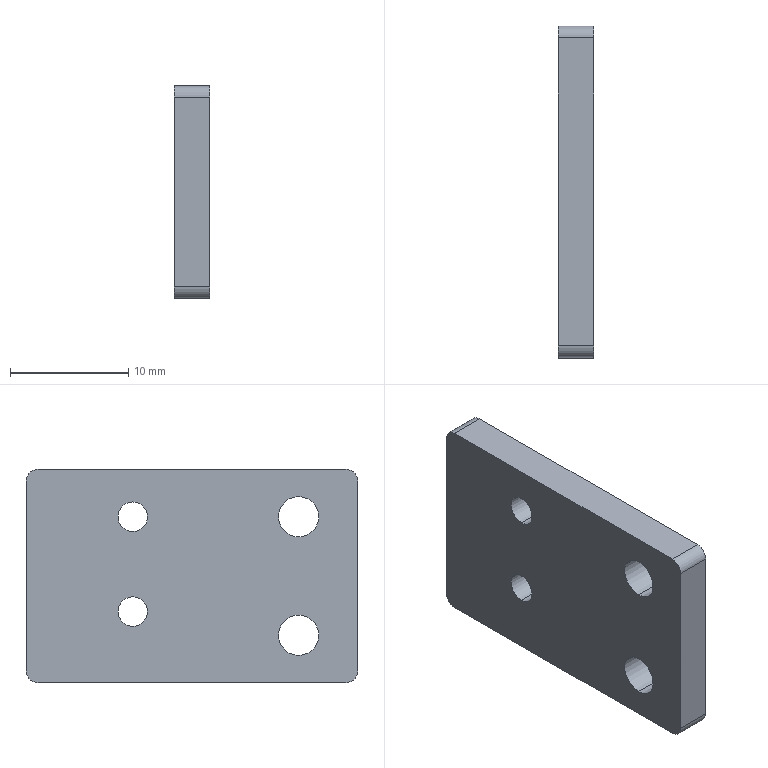Part | NX | features BREP 1 | 1 solid | 18 faces | box 3 x 28 x 18 mm | volume 1425 mm3 | cylinder 12 | plane 6 | commonest cylinder face diameters 2 x4 2.5 x4 3.4 x4
STEP:
#1=CARTESIAN_POINT('',(-3.,28.,-8.));
#2=VERTEX_POINT('',#1);
#3=CARTESIAN_POINT('',(-3.,27.,-9.));
#4=VERTEX_POINT('',#3);
#5=CARTESIAN_POINT('',(-3.,27.,-8.));
#6=DIRECTION('',(-1.,0.,0.));
#7=DIRECTION('',(0.,1.,0.));
#8=AXIS2_PLACEMENT_3D('',#5,#6,#7);
#9=CIRCLE('',#8,1.);
#10=EDGE_CURVE('',#2,#4,#9,.T.);
#11=ORIENTED_EDGE('',*,*,#10,.F.);
#12=CARTESIAN_POINT('',(0.,28.,-8.));
#13=VERTEX_POINT('',#12);
#14=CARTESIAN_POINT('',(-3.,28.,-8.));
#15=DIRECTION('',(-1.,0.,0.));
#16=VECTOR('',#15,1000.);
#17=LINE('',#14,#16);
#18=EDGE_CURVE('',#13,#2,#17,.T.);
#19=ORIENTED_EDGE('',*,*,#18,.F.);
#20=CARTESIAN_POINT('',(0.,27.,-9.));
#21=VERTEX_POINT('',#20);
#22=CARTESIAN_POINT('',(0.,27.,-8.));
#23=DIRECTION('',(1.,0.,0.));
#24=DIRECTION('',(0.,1.,0.));
#25=AXIS2_PLACEMENT_3D('',#22,#23,#24);
#26=CIRCLE('',#25,1.);
#27=EDGE_CURVE('',#21,#13,#26,.T.);
#28=ORIENTED_EDGE('',*,*,#27,.F.);
#29=CARTESIAN_POINT('',(0.,27.,-9.));
#30=DIRECTION('',(1.,0.,0.));
#31=VECTOR('',#30,1000.);
#32=LINE('',#29,#31);
#33=EDGE_CURVE('',#4,#21,#32,.T.);
#34=ORIENTED_EDGE('',*,*,#33,.F.);
#35=EDGE_LOOP('',(#11,#19,#28,#34));
#36=FACE_BOUND('',#35,.T.);
#37=CARTESIAN_POINT('',(0.,27.,-8.));
#38=DIRECTION('',(1.,0.,0.));
#39=DIRECTION('',(0.,0.,-1.));
#40=AXIS2_PLACEMENT_3D('',#37,#38,#39);
#41=CYLINDRICAL_SURFACE('',#40,1.);
#42=ADVANCED_FACE('',(#36),#41,.T.);
#43=CARTESIAN_POINT('',(-3.,27.,9.));
#44=VERTEX_POINT('',#43);
#45=CARTESIAN_POINT('',(-3.,28.,8.));
#46=VERTEX_POINT('',#45);
#47=CARTESIAN_POINT('',(-3.,27.,8.));
#48=DIRECTION('',(-1.,0.,0.));
#49=DIRECTION('',(0.,1.,0.));
#50=AXIS2_PLACEMENT_3D('',#47,#48,#49);
#51=CIRCLE('',#50,1.);
#52=EDGE_CURVE('',#44,#46,#51,.T.);
#53=ORIENTED_EDGE('',*,*,#52,.F.);
#54=CARTESIAN_POINT('',(0.,27.,9.));
#55=VERTEX_POINT('',#54);
#56=CARTESIAN_POINT('',(-3.,27.,9.));
#57=DIRECTION('',(-1.,0.,0.));
#58=VECTOR('',#57,1000.);
#59=LINE('',#56,#58);
#60=EDGE_CURVE('',#55,#44,#59,.T.);
#61=ORIENTED_EDGE('',*,*,#60,.F.);
#62=CARTESIAN_POINT('',(0.,28.,8.));
#63=VERTEX_POINT('',#62);
#64=CARTESIAN_POINT('',(0.,27.,8.));
#65=DIRECTION('',(1.,0.,0.));
#66=DIRECTION('',(0.,1.,0.));
#67=AXIS2_PLACEMENT_3D('',#64,#65,#66);
#68=CIRCLE('',#67,1.);
#69=EDGE_CURVE('',#63,#55,#68,.T.);
#70=ORIENTED_EDGE('',*,*,#69,.F.);
#71=CARTESIAN_POINT('',(0.,28.,8.));
#72=DIRECTION('',(1.,0.,0.));
#73=VECTOR('',#72,1000.);
#74=LINE('',#71,#73);
#75=EDGE_CURVE('',#46,#63,#74,.T.);
#76=ORIENTED_EDGE('',*,*,#75,.F.);
#77=EDGE_LOOP('',(#53,#61,#70,#76));
#78=FACE_BOUND('',#77,.T.);
#79=CARTESIAN_POINT('',(-3.,27.,8.));
#80=DIRECTION('',(-1.,0.,0.));
#81=DIRECTION('',(0.,0.,1.));
#82=AXIS2_PLACEMENT_3D('',#79,#80,#81);
#83=CYLINDRICAL_SURFACE('',#82,1.);
#84=ADVANCED_FACE('',(#78),#83,.T.);
#85=CARTESIAN_POINT('',(0.,0.,-8.));
#86=VERTEX_POINT('',#85);
#87=CARTESIAN_POINT('',(0.,1.,-9.));
#88=VERTEX_POINT('',#87);
#89=CARTESIAN_POINT('',(0.,1.,-8.));
#90=DIRECTION('',(1.,0.,0.));
#91=DIRECTION('',(0.,1.,0.));
#92=AXIS2_PLACEMENT_3D('',#89,#90,#91);
#93=CIRCLE('',#92,1.);
#94=EDGE_CURVE('',#86,#88,#93,.T.);
#95=ORIENTED_EDGE('',*,*,#94,.F.);
#96=CARTESIAN_POINT('',(-3.,0.,-8.));
#97=VERTEX_POINT('',#96);
#98=CARTESIAN_POINT('',(0.,0.,-8.));
#99=DIRECTION('',(1.,0.,0.));
#100=VECTOR('',#99,1000.);
#101=LINE('',#98,#100);
#102=EDGE_CURVE('',#97,#86,#101,.T.);
#103=ORIENTED_EDGE('',*,*,#102,.F.);
#104=CARTESIAN_POINT('',(-3.,1.,-9.));
#105=VERTEX_POINT('',#104);
#106=CARTESIAN_POINT('',(-3.,1.,-8.));
#107=DIRECTION('',(-1.,0.,0.));
#108=DIRECTION('',(0.,1.,0.));
#109=AXIS2_PLACEMENT_3D('',#106,#107,#108);
#110=CIRCLE('',#109,1.);
#111=EDGE_CURVE('',#105,#97,#110,.T.);
#112=ORIENTED_EDGE('',*,*,#111,.F.);
#113=CARTESIAN_POINT('',(0.,1.,-9.));
#114=DIRECTION('',(-1.,0.,0.));
#115=VECTOR('',#114,1000.);
#116=LINE('',#113,#115);
#117=EDGE_CURVE('',#88,#105,#116,.T.);
#118=ORIENTED_EDGE('',*,*,#117,.F.);
#119=EDGE_LOOP('',(#95,#103,#112,#118));
#120=FACE_BOUND('',#119,.T.);
#121=CARTESIAN_POINT('',(0.,1.,-8.));
#122=DIRECTION('',(-1.,0.,0.));
#123=DIRECTION('',(0.,0.,1.));
#124=AXIS2_PLACEMENT_3D('',#121,#122,#123);
#125=CYLINDRICAL_SURFACE('',#124,1.);
#126=ADVANCED_FACE('',(#120),#125,.T.);
#127=CARTESIAN_POINT('',(0.,1.,9.));
#128=VERTEX_POINT('',#127);
#129=CARTESIAN_POINT('',(0.,0.,8.));
#130=VERTEX_POINT('',#129);
#131=CARTESIAN_POINT('',(0.,1.,8.));
#132=DIRECTION('',(1.,0.,0.));
#133=DIRECTION('',(0.,1.,0.));
#134=AXIS2_PLACEMENT_3D('',#131,#132,#133);
#135=CIRCLE('',#134,1.);
#136=EDGE_CURVE('',#128,#130,#135,.T.);
#137=ORIENTED_EDGE('',*,*,#136,.F.);
#138=CARTESIAN_POINT('',(-3.,1.,9.));
#139=VERTEX_POINT('',#138);
#140=CARTESIAN_POINT('',(0.,1.,9.));
#141=DIRECTION('',(1.,0.,0.));
#142=VECTOR('',#141,1000.);
#143=LINE('',#140,#142);
#144=EDGE_CURVE('',#139,#128,#143,.T.);
#145=ORIENTED_EDGE('',*,*,#144,.F.);
#146=CARTESIAN_POINT('',(-3.,0.,8.));
#147=VERTEX_POINT('',#146);
#148=CARTESIAN_POINT('',(-3.,1.,8.));
#149=DIRECTION('',(-1.,0.,0.));
#150=DIRECTION('',(0.,1.,0.));
#151=AXIS2_PLACEMENT_3D('',#148,#149,#150);
#152=CIRCLE('',#151,1.);
#153=EDGE_CURVE('',#147,#139,#152,.T.);
#154=ORIENTED_EDGE('',*,*,#153,.F.);
#155=CARTESIAN_POINT('',(-3.,0.,8.));
#156=DIRECTION('',(-1.,0.,0.));
#157=VECTOR('',#156,1000.);
#158=LINE('',#155,#157);
#159=EDGE_CURVE('',#130,#147,#158,.T.);
#160=ORIENTED_EDGE('',*,*,#159,.F.);
#161=EDGE_LOOP('',(#137,#145,#154,#160));
#162=FACE_BOUND('',#161,.T.);
#163=CARTESIAN_POINT('',(0.,1.,8.));
#164=DIRECTION('',(1.,0.,0.));
#165=DIRECTION('',(0.,0.,-1.));
#166=AXIS2_PLACEMENT_3D('',#163,#164,#165);
#167=CYLINDRICAL_SURFACE('',#166,1.);
#168=ADVANCED_FACE('',(#162),#167,.T.);
#169=CARTESIAN_POINT('',(-3.,5.,-6.7));
#170=VERTEX_POINT('',#169);
#171=CARTESIAN_POINT('',(0.,5.,-6.7));
#172=VERTEX_POINT('',#171);
#173=CARTESIAN_POINT('',(-3.,5.,-6.7));
#174=DIRECTION('',(-1.,0.,0.));
#175=VECTOR('',#174,1000.);
#176=LINE('',#173,#175);
#177=EDGE_CURVE('',#170,#172,#176,.F.);
#178=ORIENTED_EDGE('',*,*,#177,.T.);
#179=CARTESIAN_POINT('',(0.,5.,-3.3));
#180=VERTEX_POINT('',#179);
#181=CARTESIAN_POINT('',(0.,5.,-5.));
#182=DIRECTION('',(-1.,0.,0.));
#183=DIRECTION('',(0.,0.,1.));
#184=AXIS2_PLACEMENT_3D('',#181,#182,#183);
#185=CIRCLE('',#184,1.7);
#186=EDGE_CURVE('',#180,#172,#185,.T.);
#187=ORIENTED_EDGE('',*,*,#186,.F.);
#188=CARTESIAN_POINT('',(-3.,5.,-3.3));
#189=VERTEX_POINT('',#188);
#190=CARTESIAN_POINT('',(-3.,5.,-3.3));
#191=DIRECTION('',(-1.,0.,0.));
#192=VECTOR('',#191,1000.);
#193=LINE('',#190,#192);
#194=EDGE_CURVE('',#189,#180,#193,.F.);
#195=ORIENTED_EDGE('',*,*,#194,.F.);
#196=CARTESIAN_POINT('',(-3.,5.,-5.));
#197=DIRECTION('',(-1.,0.,0.));
#198=DIRECTION('',(0.,0.,1.));
#199=AXIS2_PLACEMENT_3D('',#196,#197,#198);
#200=CIRCLE('',#199,1.7);
#201=EDGE_CURVE('',#189,#170,#200,.T.);
#202=ORIENTED_EDGE('',*,*,#201,.T.);
#203=EDGE_LOOP('',(#178,#187,#195,#202));
#204=FACE_BOUND('',#203,.T.);
#205=CARTESIAN_POINT('',(-3.,5.,-5.));
#206=DIRECTION('',(-1.,0.,0.));
#207=DIRECTION('',(0.,0.,1.));
#208=AXIS2_PLACEMENT_3D('',#205,#206,#207);
#209=CYLINDRICAL_SURFACE('',#208,1.7);
#210=ADVANCED_FACE('',(#204),#209,.F.);
#211=CARTESIAN_POINT('',(-3.,5.,3.3));
#212=VERTEX_POINT('',#211);
#213=CARTESIAN_POINT('',(0.,5.,3.3));
#214=VERTEX_POINT('',#213);
#215=CARTESIAN_POINT('',(-3.,5.,3.3));
#216=DIRECTION('',(-1.,0.,0.));
#217=VECTOR('',#216,1000.);
#218=LINE('',#215,#217);
#219=EDGE_CURVE('',#212,#214,#218,.F.);
#220=ORIENTED_EDGE('',*,*,#219,.T.);
#221=CARTESIAN_POINT('',(0.,5.,6.7));
#222=VERTEX_POINT('',#221);
#223=CARTESIAN_POINT('',(0.,5.,5.));
#224=DIRECTION('',(-1.,0.,0.));
#225=DIRECTION('',(0.,0.,1.));
#226=AXIS2_PLACEMENT_3D('',#223,#224,#225);
#227=CIRCLE('',#226,1.7);
#228=EDGE_CURVE('',#222,#214,#227,.T.);
#229=ORIENTED_EDGE('',*,*,#228,.F.);
#230=CARTESIAN_POINT('',(-3.,5.,6.7));
#231=VERTEX_POINT('',#230);
#232=CARTESIAN_POINT('',(-3.,5.,6.7));
#233=DIRECTION('',(-1.,0.,0.));
#234=VECTOR('',#233,1000.);
#235=LINE('',#232,#234);
#236=EDGE_CURVE('',#231,#222,#235,.F.);
#237=ORIENTED_EDGE('',*,*,#236,.F.);
#238=CARTESIAN_POINT('',(-3.,5.,5.));
#239=DIRECTION('',(-1.,0.,0.));
#240=DIRECTION('',(0.,0.,1.));
#241=AXIS2_PLACEMENT_3D('',#238,#239,#240);
#242=CIRCLE('',#241,1.7);
#243=EDGE_CURVE('',#231,#212,#242,.T.);
#244=ORIENTED_EDGE('',*,*,#243,.T.);
#245=EDGE_LOOP('',(#220,#229,#237,#244));
#246=FACE_BOUND('',#245,.T.);
#247=CARTESIAN_POINT('',(-3.,5.,5.));
#248=DIRECTION('',(-1.,0.,0.));
#249=DIRECTION('',(0.,0.,1.));
#250=AXIS2_PLACEMENT_3D('',#247,#248,#249);
#251=CYLINDRICAL_SURFACE('',#250,1.7);
#252=ADVANCED_FACE('',(#246),#251,.F.);
#253=CARTESIAN_POINT('',(-3.,19.,-4.25));
#254=VERTEX_POINT('',#253);
#255=CARTESIAN_POINT('',(0.,19.,-4.25));
#256=VERTEX_POINT('',#255);
#257=CARTESIAN_POINT('',(-3.,19.,-4.25));
#258=DIRECTION('',(-1.,0.,0.));
#259=VECTOR('',#258,1000.);
#260=LINE('',#257,#259);
#261=EDGE_CURVE('',#254,#256,#260,.F.);
#262=ORIENTED_EDGE('',*,*,#261,.T.);
#263=CARTESIAN_POINT('',(0.,19.,-1.75));
#264=VERTEX_POINT('',#263);
#265=CARTESIAN_POINT('',(0.,19.,-3.));
#266=DIRECTION('',(1.,0.,0.));
#267=DIRECTION('',(0.,1.,0.));
#268=AXIS2_PLACEMENT_3D('',#265,#266,#267);
#269=CIRCLE('',#268,1.25);
#270=EDGE_CURVE('',#256,#264,#269,.T.);
#271=ORIENTED_EDGE('',*,*,#270,.T.);
#272=CARTESIAN_POINT('',(-3.,19.,-1.75));
#273=VERTEX_POINT('',#272);
#274=CARTESIAN_POINT('',(-3.,19.,-1.75));
#275=DIRECTION('',(-1.,0.,0.));
#276=VECTOR('',#275,1000.);
#277=LINE('',#274,#276);
#278=EDGE_CURVE('',#273,#264,#277,.F.);
#279=ORIENTED_EDGE('',*,*,#278,.F.);
#280=CARTESIAN_POINT('',(-3.,19.,-3.));
#281=DIRECTION('',(-1.,0.,0.));
#282=DIRECTION('',(0.,0.,1.));
#283=AXIS2_PLACEMENT_3D('',#280,#281,#282);
#284=CIRCLE('',#283,1.25);
#285=EDGE_CURVE('',#273,#254,#284,.T.);
#286=ORIENTED_EDGE('',*,*,#285,.T.);
#287=EDGE_LOOP('',(#262,#271,#279,#286));
#288=FACE_BOUND('',#287,.T.);
#289=CARTESIAN_POINT('',(-3.,19.,-3.));
#290=DIRECTION('',(-1.,0.,0.));
#291=DIRECTION('',(0.,0.,1.));
#292=AXIS2_PLACEMENT_3D('',#289,#290,#291);
#293=CYLINDRICAL_SURFACE('',#292,1.25);
#294=ADVANCED_FACE('',(#288),#293,.F.);
#295=CARTESIAN_POINT('',(-3.,19.,3.75));
#296=VERTEX_POINT('',#295);
#297=CARTESIAN_POINT('',(0.,19.,3.75));
#298=VERTEX_POINT('',#297);
#299=CARTESIAN_POINT('',(-3.,19.,3.75));
#300=DIRECTION('',(-1.,0.,0.));
#301=VECTOR('',#300,1000.);
#302=LINE('',#299,#301);
#303=EDGE_CURVE('',#296,#298,#302,.F.);
#304=ORIENTED_EDGE('',*,*,#303,.T.);
#305=CARTESIAN_POINT('',(0.,19.,6.25));
#306=VERTEX_POINT('',#305);
#307=CARTESIAN_POINT('',(0.,19.,5.));
#308=DIRECTION('',(1.,0.,0.));
#309=DIRECTION('',(0.,1.,0.));
#310=AXIS2_PLACEMENT_3D('',#307,#308,#309);
#311=CIRCLE('',#310,1.25);
#312=EDGE_CURVE('',#298,#306,#311,.T.);
#313=ORIENTED_EDGE('',*,*,#312,.T.);
#314=CARTESIAN_POINT('',(-3.,19.,6.25));
#315=VERTEX_POINT('',#314);
#316=CARTESIAN_POINT('',(-3.,19.,6.25));
#317=DIRECTION('',(-1.,0.,0.));
#318=VECTOR('',#317,1000.);
#319=LINE('',#316,#318);
#320=EDGE_CURVE('',#315,#306,#319,.F.);
#321=ORIENTED_EDGE('',*,*,#320,.F.);
#322=CARTESIAN_POINT('',(-3.,19.,5.));
#323=DIRECTION('',(-1.,0.,0.));
#324=DIRECTION('',(0.,0.,1.));
#325=AXIS2_PLACEMENT_3D('',#322,#323,#324);
#326=CIRCLE('',#325,1.25);
#327=EDGE_CURVE('',#315,#296,#326,.T.);
#328=ORIENTED_EDGE('',*,*,#327,.T.);
#329=EDGE_LOOP('',(#304,#313,#321,#328));
#330=FACE_BOUND('',#329,.T.);
#331=CARTESIAN_POINT('',(-3.,19.,5.));
#332=DIRECTION('',(-1.,0.,0.));
#333=DIRECTION('',(0.,0.,1.));
#334=AXIS2_PLACEMENT_3D('',#331,#332,#333);
#335=CYLINDRICAL_SURFACE('',#334,1.25);
#336=ADVANCED_FACE('',(#330),#335,.F.);
#337=CARTESIAN_POINT('',(0.,28.,-9.));
#338=DIRECTION('',(0.,-1.,0.));
#339=VECTOR('',#338,1000.);
#340=LINE('',#337,#339);
#341=EDGE_CURVE('',#21,#88,#340,.T.);
#342=ORIENTED_EDGE('',*,*,#341,.T.);
#343=ORIENTED_EDGE('',*,*,#117,.T.);
#344=CARTESIAN_POINT('',(-3.,28.,-9.));
#345=DIRECTION('',(0.,-1.,0.));
#346=VECTOR('',#345,1000.);
#347=LINE('',#344,#346);
#348=EDGE_CURVE('',#4,#105,#347,.T.);
#349=ORIENTED_EDGE('',*,*,#348,.F.);
#350=ORIENTED_EDGE('',*,*,#33,.T.);
#351=EDGE_LOOP('',(#342,#343,#349,#350));
#352=FACE_BOUND('',#351,.T.);
#353=CARTESIAN_POINT('',(0.,0.,-9.));
#354=DIRECTION('',(0.,0.,-1.));
#355=DIRECTION('',(-1.,0.,0.));
#356=AXIS2_PLACEMENT_3D('',#353,#354,#355);
#357=PLANE('',#356);
#358=ADVANCED_FACE('',(#352),#357,.T.);
#359=CARTESIAN_POINT('',(-3.,28.,9.));
#360=DIRECTION('',(0.,-1.,0.));
#361=VECTOR('',#360,1000.);
#362=LINE('',#359,#361);
#363=EDGE_CURVE('',#44,#139,#362,.T.);
#364=ORIENTED_EDGE('',*,*,#363,.T.);
#365=ORIENTED_EDGE('',*,*,#144,.T.);
#366=CARTESIAN_POINT('',(0.,28.,9.));
#367=DIRECTION('',(0.,-1.,0.));
#368=VECTOR('',#367,1000.);
#369=LINE('',#366,#368);
#370=EDGE_CURVE('',#55,#128,#369,.T.);
#371=ORIENTED_EDGE('',*,*,#370,.F.);
#372=ORIENTED_EDGE('',*,*,#60,.T.);
#373=EDGE_LOOP('',(#364,#365,#371,#372));
#374=FACE_BOUND('',#373,.T.);
#375=CARTESIAN_POINT('',(0.,0.,9.));
#376=DIRECTION('',(0.,0.,-1.));
#377=DIRECTION('',(-1.,0.,0.));
#378=AXIS2_PLACEMENT_3D('',#375,#376,#377);
#379=PLANE('',#378);
#380=ADVANCED_FACE('',(#374),#379,.F.);
#381=CARTESIAN_POINT('',(-3.,28.,9.));
#382=DIRECTION('',(0.,0.,-1.));
#383=VECTOR('',#382,1000.);
#384=LINE('',#381,#383);
#385=EDGE_CURVE('',#46,#2,#384,.T.);
#386=ORIENTED_EDGE('',*,*,#385,.F.);
#387=ORIENTED_EDGE('',*,*,#75,.T.);
#388=CARTESIAN_POINT('',(0.,28.,9.));
#389=DIRECTION('',(0.,0.,-1.));
#390=VECTOR('',#389,1000.);
#391=LINE('',#388,#390);
#392=EDGE_CURVE('',#63,#13,#391,.T.);
#393=ORIENTED_EDGE('',*,*,#392,.T.);
#394=ORIENTED_EDGE('',*,*,#18,.T.);
#395=EDGE_LOOP('',(#386,#387,#393,#394));
#396=FACE_BOUND('',#395,.T.);
#397=CARTESIAN_POINT('',(-3.,28.,9.));
#398=DIRECTION('',(0.,1.,0.));
#399=DIRECTION('',(0.,0.,1.));
#400=AXIS2_PLACEMENT_3D('',#397,#398,#399);
#401=PLANE('',#400);
#402=ADVANCED_FACE('',(#396),#401,.T.);
#403=ORIENTED_EDGE('',*,*,#370,.T.);
#404=ORIENTED_EDGE('',*,*,#136,.T.);
#405=CARTESIAN_POINT('',(0.,0.,9.));
#406=DIRECTION('',(0.,0.,-1.));
#407=VECTOR('',#406,1000.);
#408=LINE('',#405,#407);
#409=EDGE_CURVE('',#130,#86,#408,.T.);
#410=ORIENTED_EDGE('',*,*,#409,.T.);
#411=ORIENTED_EDGE('',*,*,#94,.T.);
#412=ORIENTED_EDGE('',*,*,#341,.F.);
#413=ORIENTED_EDGE('',*,*,#27,.T.);
#414=ORIENTED_EDGE('',*,*,#392,.F.);
#415=ORIENTED_EDGE('',*,*,#69,.T.);
#416=EDGE_LOOP('',(#403,#404,#410,#411,#412,#413,#414,#415));
#417=FACE_BOUND('',#416,.T.);
#418=CARTESIAN_POINT('',(0.,19.,5.));
#419=DIRECTION('',(1.,0.,0.));
#420=DIRECTION('',(0.,1.,0.));
#421=AXIS2_PLACEMENT_3D('',#418,#419,#420);
#422=CIRCLE('',#421,1.25);
#423=EDGE_CURVE('',#306,#298,#422,.T.);
#424=ORIENTED_EDGE('',*,*,#423,.F.);
#425=ORIENTED_EDGE('',*,*,#312,.F.);
#426=EDGE_LOOP('',(#424,#425));
#427=FACE_BOUND('',#426,.T.);
#428=CARTESIAN_POINT('',(0.,19.,-3.));
#429=DIRECTION('',(1.,0.,0.));
#430=DIRECTION('',(0.,1.,0.));
#431=AXIS2_PLACEMENT_3D('',#428,#429,#430);
#432=CIRCLE('',#431,1.25);
#433=EDGE_CURVE('',#264,#256,#432,.T.);
#434=ORIENTED_EDGE('',*,*,#433,.F.);
#435=ORIENTED_EDGE('',*,*,#270,.F.);
#436=EDGE_LOOP('',(#434,#435));
#437=FACE_BOUND('',#436,.T.);
#438=ORIENTED_EDGE('',*,*,#228,.T.);
#439=CARTESIAN_POINT('',(0.,5.,5.));
#440=DIRECTION('',(-1.,0.,0.));
#441=DIRECTION('',(0.,0.,1.));
#442=AXIS2_PLACEMENT_3D('',#439,#440,#441);
#443=CIRCLE('',#442,1.7);
#444=EDGE_CURVE('',#214,#222,#443,.T.);
#445=ORIENTED_EDGE('',*,*,#444,.T.);
#446=EDGE_LOOP('',(#438,#445));
#447=FACE_BOUND('',#446,.T.);
#448=ORIENTED_EDGE('',*,*,#186,.T.);
#449=CARTESIAN_POINT('',(0.,5.,-5.));
#450=DIRECTION('',(-1.,0.,0.));
#451=DIRECTION('',(0.,0.,1.));
#452=AXIS2_PLACEMENT_3D('',#449,#450,#451);
#453=CIRCLE('',#452,1.7);
#454=EDGE_CURVE('',#172,#180,#453,.T.);
#455=ORIENTED_EDGE('',*,*,#454,.T.);
#456=EDGE_LOOP('',(#448,#455));
#457=FACE_BOUND('',#456,.T.);
#458=CARTESIAN_POINT('',(0.,28.,9.));
#459=DIRECTION('',(1.,0.,0.));
#460=DIRECTION('',(0.,1.,0.));
#461=AXIS2_PLACEMENT_3D('',#458,#459,#460);
#462=PLANE('',#461);
#463=ADVANCED_FACE('',(#417,#427,#437,#447,#457),#462,.T.);
#464=ORIENTED_EDGE('',*,*,#409,.F.);
#465=ORIENTED_EDGE('',*,*,#159,.T.);
#466=CARTESIAN_POINT('',(-3.,0.,9.));
#467=DIRECTION('',(0.,0.,-1.));
#468=VECTOR('',#467,1000.);
#469=LINE('',#466,#468);
#470=EDGE_CURVE('',#147,#97,#469,.T.);
#471=ORIENTED_EDGE('',*,*,#470,.T.);
#472=ORIENTED_EDGE('',*,*,#102,.T.);
#473=EDGE_LOOP('',(#464,#465,#471,#472));
#474=FACE_BOUND('',#473,.T.);
#475=CARTESIAN_POINT('',(0.,0.,9.));
#476=DIRECTION('',(0.,-1.,0.));
#477=DIRECTION('',(0.,0.,-1.));
#478=AXIS2_PLACEMENT_3D('',#475,#476,#477);
#479=PLANE('',#478);
#480=ADVANCED_FACE('',(#474),#479,.T.);
#481=ORIENTED_EDGE('',*,*,#470,.F.);
#482=ORIENTED_EDGE('',*,*,#153,.T.);
#483=ORIENTED_EDGE('',*,*,#363,.F.);
#484=ORIENTED_EDGE('',*,*,#52,.T.);
#485=ORIENTED_EDGE('',*,*,#385,.T.);
#486=ORIENTED_EDGE('',*,*,#10,.T.);
#487=ORIENTED_EDGE('',*,*,#348,.T.);
#488=ORIENTED_EDGE('',*,*,#111,.T.);
#489=EDGE_LOOP('',(#481,#482,#483,#484,#485,#486,#487,#488));
#490=FACE_BOUND('',#489,.T.);
#491=ORIENTED_EDGE('',*,*,#327,.F.);
#492=CARTESIAN_POINT('',(-3.,19.,5.));
#493=DIRECTION('',(-1.,0.,0.));
#494=DIRECTION('',(0.,0.,1.));
#495=AXIS2_PLACEMENT_3D('',#492,#493,#494);
#496=CIRCLE('',#495,1.25);
#497=EDGE_CURVE('',#296,#315,#496,.T.);
#498=ORIENTED_EDGE('',*,*,#497,.F.);
#499=EDGE_LOOP('',(#491,#498));
#500=FACE_BOUND('',#499,.T.);
#501=ORIENTED_EDGE('',*,*,#285,.F.);
#502=CARTESIAN_POINT('',(-3.,19.,-3.));
#503=DIRECTION('',(-1.,0.,0.));
#504=DIRECTION('',(0.,0.,1.));
#505=AXIS2_PLACEMENT_3D('',#502,#503,#504);
#506=CIRCLE('',#505,1.25);
#507=EDGE_CURVE('',#254,#273,#506,.T.);
#508=ORIENTED_EDGE('',*,*,#507,.F.);
#509=EDGE_LOOP('',(#501,#508));
#510=FACE_BOUND('',#509,.T.);
#511=ORIENTED_EDGE('',*,*,#243,.F.);
#512=CARTESIAN_POINT('',(-3.,5.,5.));
#513=DIRECTION('',(-1.,0.,0.));
#514=DIRECTION('',(0.,0.,1.));
#515=AXIS2_PLACEMENT_3D('',#512,#513,#514);
#516=CIRCLE('',#515,1.7);
#517=EDGE_CURVE('',#212,#231,#516,.T.);
#518=ORIENTED_EDGE('',*,*,#517,.F.);
#519=EDGE_LOOP('',(#511,#518));
#520=FACE_BOUND('',#519,.T.);
#521=ORIENTED_EDGE('',*,*,#201,.F.);
#522=CARTESIAN_POINT('',(-3.,5.,-5.));
#523=DIRECTION('',(-1.,0.,0.));
#524=DIRECTION('',(0.,0.,1.));
#525=AXIS2_PLACEMENT_3D('',#522,#523,#524);
#526=CIRCLE('',#525,1.7);
#527=EDGE_CURVE('',#170,#189,#526,.T.);
#528=ORIENTED_EDGE('',*,*,#527,.F.);
#529=EDGE_LOOP('',(#521,#528));
#530=FACE_BOUND('',#529,.T.);
#531=CARTESIAN_POINT('',(-3.,28.,9.));
#532=DIRECTION('',(1.,0.,0.));
#533=DIRECTION('',(0.,1.,0.));
#534=AXIS2_PLACEMENT_3D('',#531,#532,#533);
#535=PLANE('',#534);
#536=ADVANCED_FACE('',(#490,#500,#510,#520,#530),#535,.F.);
#537=ORIENTED_EDGE('',*,*,#423,.T.);
#538=ORIENTED_EDGE('',*,*,#303,.F.);
#539=ORIENTED_EDGE('',*,*,#497,.T.);
#540=ORIENTED_EDGE('',*,*,#320,.T.);
#541=EDGE_LOOP('',(#537,#538,#539,#540));
#542=FACE_BOUND('',#541,.T.);
#543=CARTESIAN_POINT('',(-3.,19.,5.));
#544=DIRECTION('',(-1.,0.,0.));
#545=DIRECTION('',(0.,0.,1.));
#546=AXIS2_PLACEMENT_3D('',#543,#544,#545);
#547=CYLINDRICAL_SURFACE('',#546,1.25);
#548=ADVANCED_FACE('',(#542),#547,.F.);
#549=ORIENTED_EDGE('',*,*,#433,.T.);
#550=ORIENTED_EDGE('',*,*,#261,.F.);
#551=ORIENTED_EDGE('',*,*,#507,.T.);
#552=ORIENTED_EDGE('',*,*,#278,.T.);
#553=EDGE_LOOP('',(#549,#550,#551,#552));
#554=FACE_BOUND('',#553,.T.);
#555=CARTESIAN_POINT('',(-3.,19.,-3.));
#556=DIRECTION('',(-1.,0.,0.));
#557=DIRECTION('',(0.,0.,1.));
#558=AXIS2_PLACEMENT_3D('',#555,#556,#557);
#559=CYLINDRICAL_SURFACE('',#558,1.25);
#560=ADVANCED_FACE('',(#554),#559,.F.);
#561=ORIENTED_EDGE('',*,*,#444,.F.);
#562=ORIENTED_EDGE('',*,*,#219,.F.);
#563=ORIENTED_EDGE('',*,*,#517,.T.);
#564=ORIENTED_EDGE('',*,*,#236,.T.);
#565=EDGE_LOOP('',(#561,#562,#563,#564));
#566=FACE_BOUND('',#565,.T.);
#567=CARTESIAN_POINT('',(-3.,5.,5.));
#568=DIRECTION('',(-1.,0.,0.));
#569=DIRECTION('',(0.,0.,1.));
#570=AXIS2_PLACEMENT_3D('',#567,#568,#569);
#571=CYLINDRICAL_SURFACE('',#570,1.7);
#572=ADVANCED_FACE('',(#566),#571,.F.);
#573=ORIENTED_EDGE('',*,*,#454,.F.);
#574=ORIENTED_EDGE('',*,*,#177,.F.);
#575=ORIENTED_EDGE('',*,*,#527,.T.);
#576=ORIENTED_EDGE('',*,*,#194,.T.);
#577=EDGE_LOOP('',(#573,#574,#575,#576));
#578=FACE_BOUND('',#577,.T.);
#579=CARTESIAN_POINT('',(-3.,5.,-5.));
#580=DIRECTION('',(-1.,0.,0.));
#581=DIRECTION('',(0.,0.,1.));
#582=AXIS2_PLACEMENT_3D('',#579,#580,#581);
#583=CYLINDRICAL_SURFACE('',#582,1.7);
#584=ADVANCED_FACE('',(#578),#583,.F.);
#585=CLOSED_SHELL('',(#42,#84,#126,#168,#210,#252,#294,#336,#358,#380,#402,#463,#480,#536,#548,#560,#572,#584));
#586=MANIFOLD_SOLID_BREP('',#585);
#587=(LENGTH_UNIT()NAMED_UNIT(*)SI_UNIT(.MILLI.,.METRE.));
#588=UNCERTAINTY_MEASURE_WITH_UNIT(LENGTH_MEASURE(0.00001),#587,'','');
#589=(NAMED_UNIT(*)PLANE_ANGLE_UNIT()SI_UNIT($,.RADIAN.));
#590=(NAMED_UNIT(*)SI_UNIT($,.STERADIAN.)SOLID_ANGLE_UNIT());
#591=(GEOMETRIC_REPRESENTATION_CONTEXT(3)GLOBAL_UNCERTAINTY_ASSIGNED_CONTEXT((#588))GLOBAL_UNIT_ASSIGNED_CONTEXT((#587,#589,#590))REPRESENTATION_CONTEXT('',''));
#592=ADVANCED_BREP_SHAPE_REPRESENTATION('',(#586),#591);